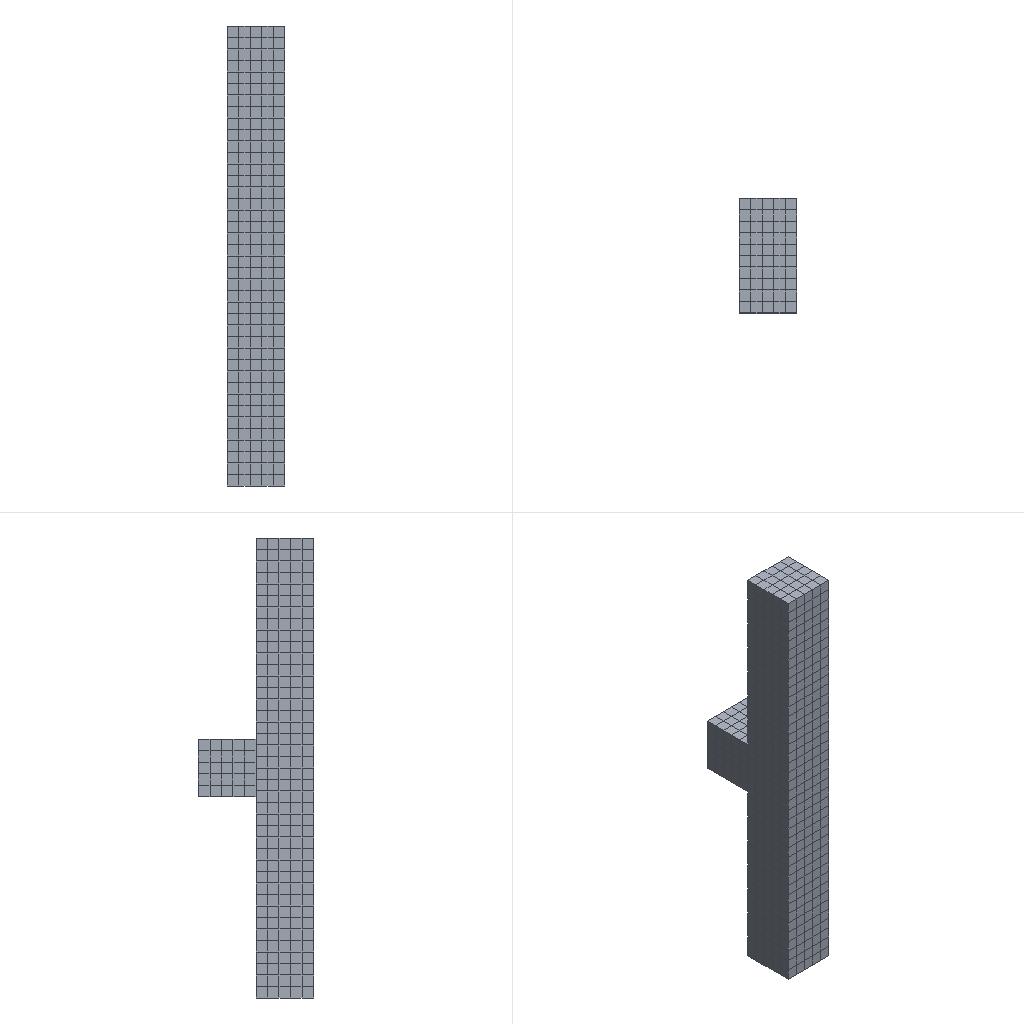Simulation study | ansys workbench
Set-up summary:
category,name,step,type,value,unit,region
solver,ansys_workbench
units,mm-N-s-tonne (MPa),,stated,"/units,MPA"
analysis,LS1,,transient
load_step,LS1,LS1,transient,time=1
mesh,nodes,,,6132
mesh,elements,,,1600
element_type,SOLID186,,,1125
element_type,TARGE170,,,225
element_type,CONTA174,,,225
element_type,SURF154,,,25
material,tansuxing,,E,210000,tonne s^-2 mm^-1
material,tansuxing,,nu,0.3
material,tansuxing,,density,7.85e-09,tonne mm^-3
material,tansuxing,,behaviors,"plastic; tb plas,BISO"
material,new123,,E,210000,tonne s^-2 mm^-1
material,new123,,nu,0.3
material,new123,,density,7.85e-09,tonne mm^-3
load,Define Pressure Vector Using Surface Effect Elements,LS1,surface-effect pres face 2,-60,,SURF154 #5
bc,Fixed Supports,model,fixed,[dofs=ALL],,_FIXEDSU
bc,Constant Zero Displacement X,model,fixed,[dofs=UX],,_DISPZEROUX
bc,Set Displacements,LS1,prescribed uz,5 [dofs=UZ],,_CM47UZ_ZP
contact,Frictional - rec To quad,,standard (frictionless/frictional),friction=0.15; element=CONTA174
named_set,_FIXEDSU,,node,192
named_set,_DISPZEROUX,,node,96
named_set,_CM47UZ_ZP,,node,96
Ansys APDL input file, long lists of numbers shortened:
/batch
/config,noeldb,1     ! force off writing results to database
*get,_wallstrt,active,,time,wall
! ANSYS input file written by Workbench version 2023 R1
! File used for geometry attach:
/title,E1.7.4--Transient (A5)
! ****** Begin Custom Load Command Snippet ******
/COM, ACT Extensions:
/COM,     LSDYNA, 2023.1
/COM,/COM,     ANSYSMotion, 2023.1
/COM,
! ****** End   Custom Load Command Snippet ******
*DIM,_wb_ProjectScratch_dir,string,248
_wb_ProjectScratch_dir(1) = ''
*DIM,_wb_SolverFiles_dir,string,248
_wb_SolverFiles_dir(1) = ''
*DIM,_wb_userfiles_dir,string,248
_wb_userfiles_dir(1) = ''
/com,--- Data in consistent NMM units. See Solving Units in the help system for more information.
/units,MPA
/nopr
/wb,file,start              !  signify a WB generated input file
/prep7
! Turn off shape checking because checks already performed inside WB mesher.
! See help system for more information.
SHPP,OFF,,NOWARN
/nolist
etcon,set             ! allow ANSYS to choose best KEYOP's for 180x elements, resets any applicable keyopt to MAPDL defaults
/com,*********** Nodes for the whole assembly ***********
nblock,3,,6745
(1i9,3e20.9e3)
        1     8.000000000E+00     1.800000000E+01     3.700000000E+01
! (6131 more lines like these left out)
-1
/wb,elem,start            !  set before creation of elements
/com,*********** Elements for Body 1 "rec" ***********
et,1,186
keyo,1,2,1          ! set full integration on SOLID186
eblock,19,solid,,1000
(19i9)
        1        1        1        1        0        0        0        0       20        0      126      757     2016     2009     1813     1536     2029     2008     2007
! (1999 more lines like these left out)
-1
/com,*********** Elements for Body 2 "quad" ***********
et,2,186
keyo,2,2,1          ! set full integration on SOLID186
eblock,19,solid,,125
(19i9)
        2        2        2        2        0        0        0        0       20        0        1        1      147      168      197       80      166      167      213
! (249 more lines like these left out)
-1
/wb,elem,end               !  done creating elements
/com,*********** Send User Defined Coordinate System(s) ***********
csys,0
toffst,273.15,  ! Temperature offset from absolute zero
/com,*********** Set Reference Temperature ***********
tref,22.
/wb,mat,start              !  starting to send materials
/com,*********** Send Materials ***********
MP,DENS,1,7.85e-09,	! tonne mm^-3
MP,EX,1,210000,	! tonne s^-2 mm^-1
MP,NUXY,1,0.3,
TB,PLAS,1,1,,BISO
TBDATA,1,300,100000
MP,DENS,2,7.85e-09,	! tonne mm^-3
MP,EX,2,210000,	! tonne s^-2 mm^-1
MP,NUXY,2,0.3,
/wb,mat,end                !  done sending materials
!************************* Model Summary ********************
!rec,	tansuxing,	matid,	1
!quad,	new123,	matid,	2
!************************* End Model Summary ********************
! get the diagonal of the bounding box. Needed later for other things
*get,_xmin,node,,mnloc,x
*get,_ymin,node,,mnloc,y
*get,_zmin,node,,mnloc,z
*get,_xmax,node,,mxloc,x
*get,_ymax,node,,mxloc,y
*get,_zmax,node,,mxloc,z
_ASMDIAG=(_xmax-_xmin)*(_xmax-_xmin)+(_ymax-_ymin)*(_ymax-_ymin)+(_zmax-_zmin)*(_zmax-_zmin)
_ASMDIAG=SQRT(_ASMDIAG)
/wb,contact,start          !  starting to send contact
/com,*********** Create Contact "Frictional - rec To quad" ***********
/com,            Real Constant Set For Above Contact Is 4 & 3
*set,tid,4
*set,cid,3
r,tid
r,cid
et,tid,170
et,cid,174
eblock,10,,,200
(15i9)
     2126        4        4        4        0     2037     2038     1731     1732     5786     5221     5220     5223
! (199 more lines like these left out)
-1
eblock,10,,,200
(15i9)
     2326        3        3        3        0     2037     2038     1731     1732     5786     5221     5220     5223
! (199 more lines like these left out)
-1
eblock,10,,,25
(15i9)
     2526        3        4        3        0      106       81       97      105      500      499      538      555
! (24 more lines like these left out)
-1
eblock,10,,,25
(15i9)
     2551        4        3        4        0      106       81       97      105      500      499      538      555
! (24 more lines like these left out)
-1
keyo,cid,8,2               ! auto create asymmetric contact (from Program Controlled setting)
keyo,cid,10,0              ! adjust contact stiffness each NR iteration
keyo,cid,12,0              ! standard contact
mp,mu,cid,0.15      ! unitless
keyo,cid,18,0              ! finite small sliding
keyo,cid,2,0               ! augmented Lagrange (from Program Controlled setting)
keyo,cid,4,0               ! on Gauss point (from Program Controlled setting)
keyo,cid,9,0               ! use real geometry with stepped effects
keyo,cid,7,1               ! Automatic Bisection
rmod,tid,3,1.       ! FKN
rmod,tid,5,0.       ! ICONT
rmod,tid,6,0.       ! PINB
rmod,tid,10,0.      ! CNOF
rmod,tid,12,0.      ! FKT
rmod,tid,36,31      ! WB DSID
rmod,cid,3,1.       ! FKN
rmod,cid,5,0.       ! ICONT
rmod,cid,6,0.       ! PINB
rmod,cid,10,0.      ! CNOF
rmod,cid,12,0.      ! FKT
rmod,cid,36,31      ! WB DSID
nsel,all
esel,all
/wb,contact,end            !  done creating contacts
/golist
/wb,load,start             !  starting to send loads
/com,*********** Fixed Supports ***********
CMBLOCK,_FIXEDSU,NODE,      192
(8i10)
      1732      1733      1734      1735      1736      1737      1777      1778
! (23 more lines like these left out)
cmsel,s,_FIXEDSU
d,all,all
nsel,all
/com,******* Constant Zero Displacement X *******
CMBLOCK,_DISPZEROUX,NODE,       96
(8i10)
        97        98        99       100       105       111       137       138
! (11 more lines like these left out)
cmsel,s,_DISPZEROUX
d,all,ux,0
nsel,all
/com,*********** Define Pressure Vector Using Surface Effect Elements ***********
local,12,0,0.,0.,0.,0.,0.,0.
csys,0
et,5,154
mat,5
eblock,10,,,25
(15i9)
     2576        5        5        5       12      213       80      166      167      496      495      676      678
! (24 more lines like these left out)
-1
esel,s,type,,5
keyop,5,2,1                ! Apply load in local coordinate system
keyop,5,7,0                ! Use deformed area for application of load
esel,all
/com,*********** Create Displacement Tables and Functions ******
*DIM,_loadvari47zp,TABLE,2,1,1,TIME
! Time values
*TAXIS,_loadvari47zp(1),1,0.,1.
! Load values
_loadvari47zp(1,1,1) = 0.
_loadvari47zp(2,1,1) = 5.
*DIM,_loadvari47zn,TABLE,2,1,1,TIME
! Time values
*TAXIS,_loadvari47zn(1),1,0.,1.
! Load values
_loadvari47zn(1,1,1) = 0.
_loadvari47zn(2,1,1) = -5.
tblist
/gst,on,on
fini
*get,_numnode,node,0,count
*get,_numelem,elem,0,count
*get, _MAXELEMNUM, elem, 0, NUM, MAX
*get, _MAXNODENUM, node, 0, NUM, MAX
*get, _MAXELEMTYPE, etyp, 0, NUM, MAX
*get, _MAXREALCONST, rcon, 0, NUM, MAX
/go
/wb,load,end               !  done creating loads
/com,--- Number of total nodes = %_numnode%
/com,--- Number of contact elements = 475
/com,--- Number of spring elements = 0
/com,--- Number of bearing elements = 0
/com,--- Number of solid elements = 1125
/com,--- Number of condensed parts = 0
/com,--- Number of total elements = %_numelem%
*get,_wallbsol,active,,time,wall
/com,****************************************************************************
/com,*************************    SOLUTION       ********************************
/com,****************************************************************************
/solu
antype,4                   ! transient analysis
nlgeom,on                  ! Turn on Large Deformation Effects
kbc,1                      ! stepped BC's
_thickRatio=  1     ! Ratio of thick parts in the model
eqsl,pcg,1e-8,,,,,,1
cntr,print,1               ! print out contact info and also make no initial contact an error
trnopt,full,,,,,hht        ! HHT time integration method
tintp, mosp			! Choose transient integration settings for moderate speed application
nldiag,cont,iter           ! print out contact info each equilibrium iteration
rescontrol,define,last,last,,dele	   ! Program Controlled
/com,****************************************************
/com,******************* SOLVE FOR LS 1 OF 1 ****************
esel,s,type,,5
nsle
sfe,all,1,pres,1,0.
sfe,all,2,pres,1,-60.
sfe,all,3,pres,1,0.
nsel,all
esel,all
/com,*** Set Displacements ***
CMBLOCK,_CM47UZ_ZP,NODE,       96
(8i10)
        97        98        99       100       105       111       137       138
! (11 more lines like these left out)
cmsel,s,_CM47UZ_ZP
d,all,uz,%_loadvari47zp%
nsel,all
/com,*** Component For All Non-Zero UZ Displacements ***
cmsel,s,_CM47uz_zp
cm,_DISPNONZEROUZ,NODE
nsel,all
/nopr
/gopr
autots,off                 ! User turned off automatic time stepping
deltim,4.e-002,4.e-002,4.e-002
time,1.
timint,on                  ! Turn on time integration effects
outres,erase
outres,all,none
outres,nsol,all,
outres,rsol,all
outres,eangl,all
outres,etmp,all
outres,veng,all
outres,strs,all,
outres,epel,all,
outres,eppl,all,
outres,cont,all,
outres,v,all,
outres,a,all,
! *********** WB SOLVE COMMAND ***********
! check interactive state
*get,ANSINTER_,active,,int
*if,ANSINTER_,ne,0,then
/eof
*endif
solve
/com *************** Write FE CONNECTORS *********
CEWRITE,file,ce,,INTE
/com,****************************************************
/com,*************** FINISHED SOLVE FOR LS 1 *************
*get,_wallasol,active,,time,wall
/nopr
*get,_numnode,node,0,count
*get,_numelem,elem,0,count
*get, _MAXELEMNUM, elem, 0, NUM, MAX
*get, _MAXNODENUM, node, 0, NUM, MAX,,,INTERNAL
*get, _MAXELEMTYPE, etyp, 0, NUM, MAX
*get, _MAXREALCONST, rcon, 0, NUM, MAX
*get,_NSOLTHREADS,active,0,ntfs
*get,_NSOLPROCESSES,active,0,npfs
/gopr
*get,_PCGITER,active,,solu,cgiter
/post1
xmlo,ENCODING,ISO-8859-1
xmlo,parm
/xml,parm,xml
fini
/gopr
*get,_walldone,active,,time,wall
_preptime=(_wallbsol-_wallstrt)*3600
_solvtime=(_wallasol-_wallbsol)*3600
_posttime=(_walldone-_wallasol)*3600
_totaltim=(_walldone-_wallstrt)*3600
*get,_dlbratio,active,0,solu,dlbr
*get,_combtime,active,0,solu,comb
*get,_ssmode,active,0,solu,ssmm
*get,_ndofs,active,0,solu,ndof
/com,--- Total number of nodes = %_numnode%
/com,--- Total number of elements = %_numelem%
/com,--- Element load balance ratio = %_dlbratio%
/com,--- Time to combine distributed files = %_combtime%
/com,--- Sparse memory mode = %_ssmode%
/com,--- Number of DOF = %_ndofs%
/wb,file,end               ! done with WB generated input
Results summary:
result,analyses[0].index,,,1
result,analyses[0].system,,,SYS
result,analyses[0].deck,,,deck.dat
result,analyses[0].solve_status,,,completed
result,analyses[0].analysis_type,,,static
result,analyses[0].physics,,,mechanical
result,analyses[0].unit_system,,,"NMM: mm, ton, N, s, mV, mA, degC"
result,analyses[0].n_sets,,,25
result,analyses[0].load_steps[0].set,set=25,,25
result,analyses[0].load_steps[0].time_or_freq,set=25,,1
result,analyses[0].load_steps[0].max_displacement_magnitude,set=25,,5.003
result,analyses[0].load_steps[0].max_von_mises_nodal,set=25,,326.657
result,analyses[0].load_steps[0].reaction_force_sum_xyz[1],set=25,,-5.04831e-09
result,analyses[0].load_steps[0].reaction_force_sum_xyz[2],set=25,,6000.6
result,analyses[0].load_steps[0].reaction_force_sum_xyz[3],set=25,,1.611
result,geometry_export[0][0],,,.step
result,geometry_export[0][1],,,ok
result,geometry_export[0][2],,,2